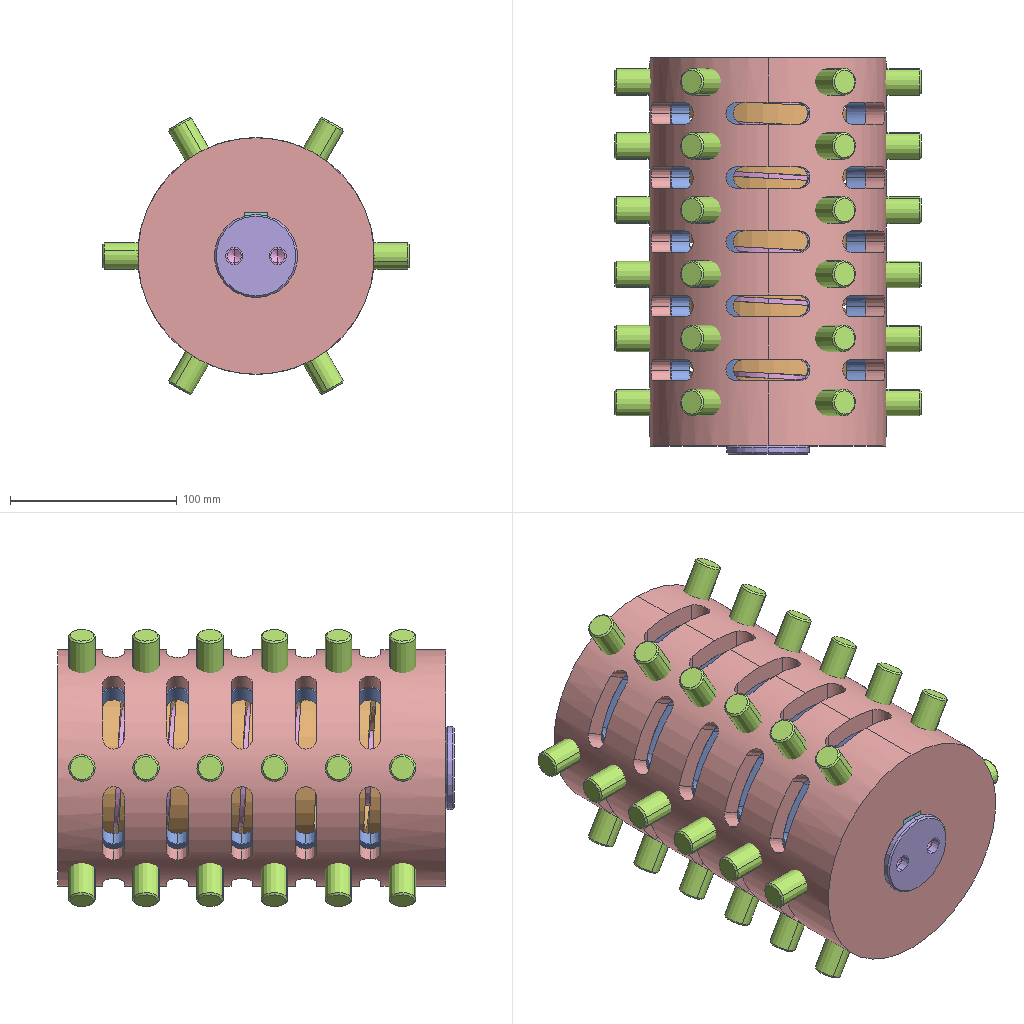Assembly | SolidWorks | 9 different items | 44 placed | box 184 x 238 x 166 mm
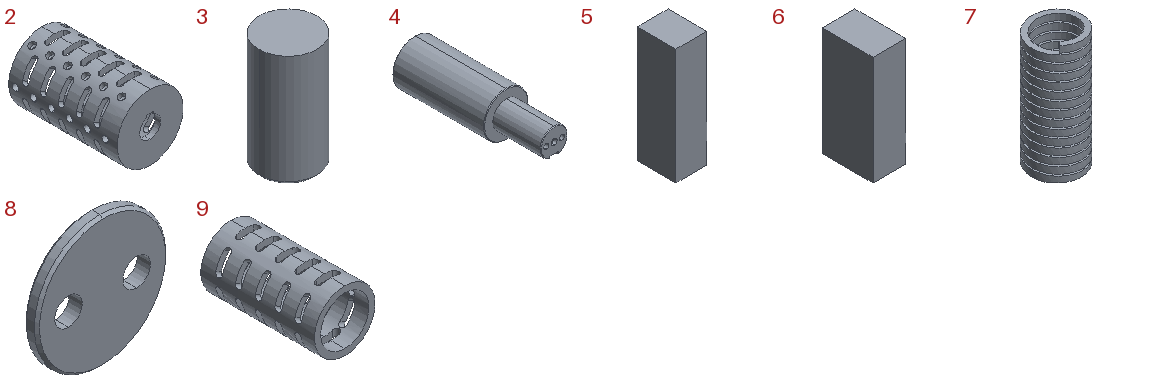Parts list (item | name | quantity | size | volume | features):
1 | B440L0101 Socket Head Cap Screw M10×25(fully threaded)stainless steel304 GB.T 70.1 | x1 | - | - | -
2 | - | x1 | 142 x 233 x 142 mm | 962955 mm3 | features CirPattern 2, ICE 2, LPattern 2, 3DProfileFeature 1, Extrusion 1, HoleWzd 1
3 | - | x36 | 16 x 16 x 31 mm | 6209 mm3 | features Chamfer 1, Extrusion 1
4 | - | x1 | 74 x 233 x 74 mm | 776364 mm3 | features ICE 3, 3DProfileFeature 2, Chamfer 2, Fillet 2, HoleWzd 2, Extrusion 1
5 | - | x1 | 8 x 10 x 30 mm | 2400 mm3 | features Extrusion 1
6 | - | x1 | 9 x 14 x 30 mm | 3780 mm3 | features Extrusion 1
7 | - | x1 | 94 x 94 x 220.999 mm | 451222 mm3 | features ICE 2, Helix 1, Sweep 1
8 | - | x1 | 50 x 5 x 50 mm | 8797 mm3 | features Chamfer 1, Extrusion 1
9 | - | x1 | 118 x 221 x 118 mm | 679782 mm3 | features CirPattern 1, Extrusion 1, ICE 1, LPattern 1
Mates (type | each side: item.copy, entity, surface, feature):
Coincident | 2.1 plane | assembly plane | 3 times
Concentric | 2.1 face cylinder CirPattern2 | 3.1 face cylinder Boss-Extrude1
Coincident | 2.1 edge | 3.1 face plane Boss-Extrude1
Concentric | 2.1 face cylinder Boss-Extrude1 | 9.1 face cylinder Boss-Extrude1
Concentric | 2.1 face cylinder Boss-Extrude2 | 4.1 face cylinder Boss-Extrude1
Parallel | 2.1 face plane Boss-Extrude2 | 4.1 face plane Boss-Extrude1
Coincident | 2.1 face plane LPattern1 | 9.1 face plane LPattern1
Coincident | 4.1 face plane Boss-Extrude1 | 6.1 face plane Boss-Extrude1 | 3 times
Concentric | 9.1 face cylinder Boss-Extrude1 | 7.1 select_type:24
Coincident | 9.1 face plane Boss-Extrude1 | 7.1 plane
Coincident | 2.1 face plane Boss-Extrude1 | 4.1 face plane Boss-Extrude1
Concentric | 4.1 face cylinder M10 Tapped Hole1 | 8.1 face cylinder Boss-Extrude1 | 2 times
Coincident | 4.1 face plane Boss-Extrude1 | 8.1 face plane Boss-Extrude1
Coincident | 7.1 plane | assembly plane
Coincident | 7.1 face plane Cut-Extrude2 | 5.1 face plane Boss-Extrude1 | 2 times
Coincident | 7.1 face plane Cut-Extrude1 | 5.1 face plane Boss-Extrude1